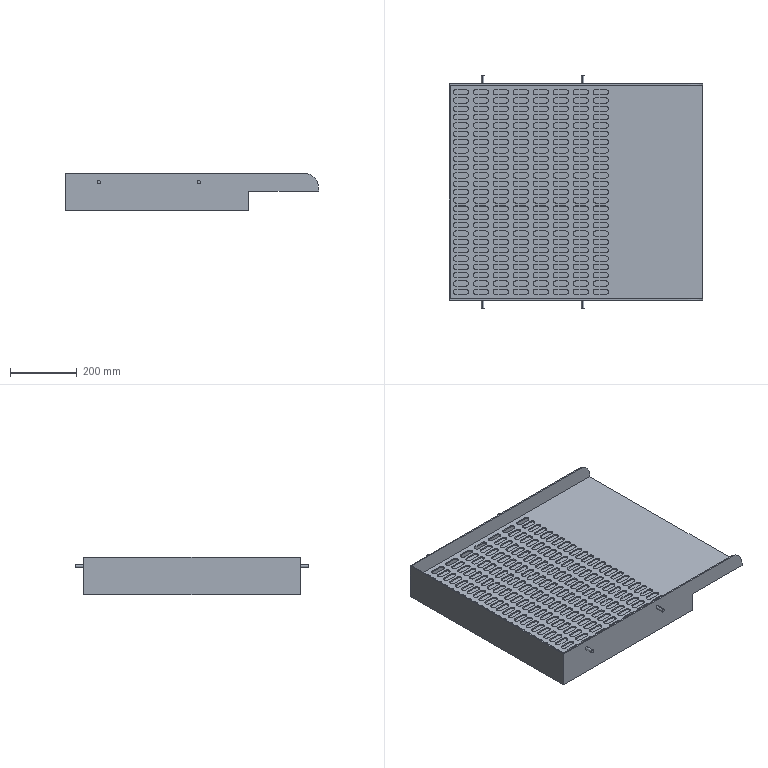Part | SolidWorks | features ICE 11, LPattern 2, Extrusion 1, Fillet 1 | 1 solid | 1049 faces | box 760 x 700 x 113 mm | volume 5573180 mm3 | cylinder 614 | plane 435 | commonest cylinder face diameters 16 x600 10 x12 90 x2